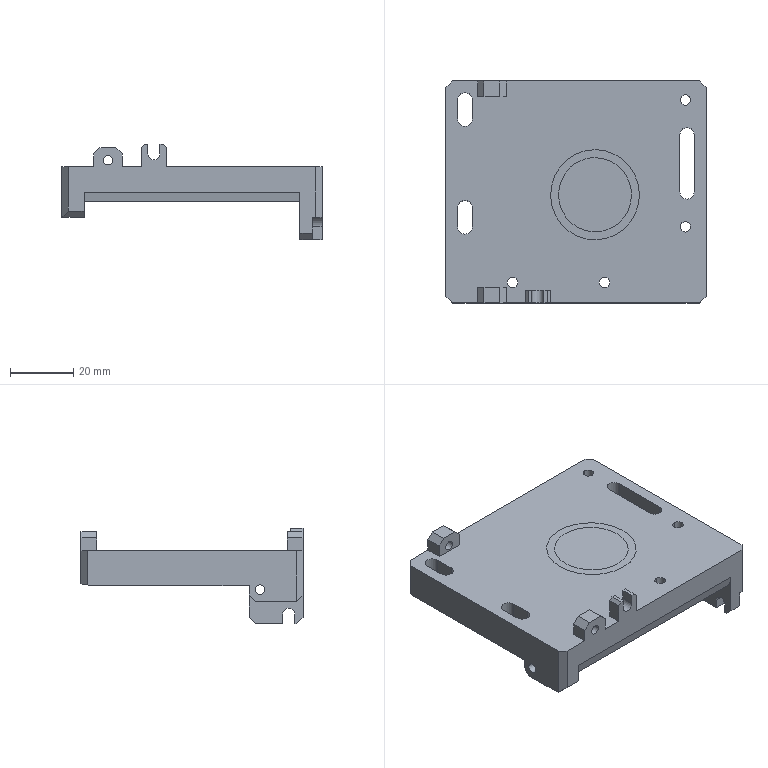NC program | NX | posted with a generic post | part box 82 x 70 x 30 mm
Lines 1 to 2118 of 5501, first 2049 of 2112 lines:
N10 G17 G21 G94 G90
(FLOOR_WALL_COPY , TOOL : D10JING)
N12 T11 M6
N14 G54
N16 G17 G0 G90 X-46. Y40.997 B0. C0. S9500 M3
N18 G43 Z30. H11
N20 Z7.5
N22 G94 G1 Z4.5 F1250.
N24 X-40.
N26 X40.
N28 Y36.122
N30 X-40.
N32 Y31.247
N34 X40.
N36 Y26.373
N38 X-40.
N40 Y21.498
N42 X40.
N44 Y16.623
N46 X-40.
N48 Y11.748
N50 X40.
N52 Y6.873
N54 X-40.
N56 Y1.999
N58 X40.
N60 Y-2.876
N62 X-40.
N64 Y-7.751
N66 X40.
N68 Y-12.626
N70 X-40.
N72 Y-17.501
N74 X40.
N76 Y-22.376
N78 X-40.
N80 Y-27.25
N82 X40.
N84 Y-32.125
N86 X-40.
N88 Y-37.
N90 X40.
N92 X46.
N94 Z7.5
N96 G0 Z30.
N98 X-46. Y40.997
N100 Z7.
N102 G1 Z4.
N104 X-40.
N106 X40.
N108 Y36.122
N110 X-40.
N112 Y31.247
N114 X40.
N116 Y26.373
N118 X-40.
N120 Y21.498
N122 X40.
N124 Y16.623
N126 X-40.
N128 Y11.748
N130 X40.
N132 Y6.873
N134 X-40.
N136 Y1.999
N138 X40.
N140 Y-2.876
N142 X-40.
N144 Y-7.751
N146 X40.
N148 Y-12.626
N150 X-40.
N152 Y-17.501
N154 X40.
N156 Y-22.376
N158 X-40.
N160 Y-27.25
N162 X40.
N164 Y-32.125
N166 X-40.
N168 Y-37.
N170 X40.
N172 X46.
N174 Z7.
N176 G0 Z30.
N178 X-46. Y40.997
N180 Z6.5
N182 G1 Z3.5
N184 X-40.
N186 X40.
N188 Y36.122
N190 X-40.
N192 Y31.247
N194 X40.
N196 Y26.373
N198 X-40.
N200 Y21.498
N202 X40.
N204 Y16.623
N206 X-40.
N208 Y11.748
N210 X40.
N212 Y6.873
N214 X-40.
N216 Y1.999
N218 X40.
N220 Y-2.876
N222 X-40.
N224 Y-7.751
N226 X40.
N228 Y-12.626
N230 X-40.
N232 Y-17.501
N234 X40.
N236 Y-22.376
N238 X-40.
N240 Y-27.25
N242 X40.
N244 Y-32.125
N246 X-40.
N248 Y-37.
N250 X40.
N252 X46.
N254 Z6.5
N256 G0 Z30.
N258 X-46. Y40.997
N260 Z6.
N262 G1 Z3.
N264 X-40.
N266 X40.
N268 Y36.122
N270 X-40.
N272 Y31.247
N274 X40.
N276 Y26.373
N278 X-40.
N280 Y21.498
N282 X40.
N284 Y16.623
N286 X-40.
N288 Y11.748
N290 X40.
N292 Y6.873
N294 X-40.
N296 Y1.999
N298 X40.
N300 Y-2.876
N302 X-40.
N304 Y-7.751
N306 X40.
N308 Y-12.626
N310 X-40.
N312 Y-17.501
N314 X40.
N316 Y-22.376
N318 X-40.
N320 Y-27.25
N322 X40.
N324 Y-32.125
N326 X-40.
N328 Y-37.
N330 X40.
N332 X46.
N334 Z6.
N336 G0 Z30.
N338 X-46. Y40.997
N340 Z5.5
N342 G1 Z2.5
N344 X-40.
N346 X40.
N348 Y36.122
N350 X-40.
N352 Y31.247
N354 X40.
N356 Y26.373
N358 X-40.
N360 Y21.498
N362 X40.
N364 Y16.623
N366 X-40.
N368 Y11.748
N370 X40.
N372 Y6.873
N374 X-40.
N376 Y1.999
N378 X40.
N380 Y-2.876
N382 X-40.
N384 Y-7.751
N386 X40.
N388 Y-12.626
N390 X-40.
N392 Y-17.501
N394 X40.
N396 Y-22.376
N398 X-40.
N400 Y-27.25
N402 X40.
N404 Y-32.125
N406 X-40.
N408 Y-37.
N410 X40.
N412 X46.
N414 Z5.5
N416 G0 Z30.
N418 X-46. Y40.997
N420 Z5.
N422 G1 Z2.
N424 X-40.
N426 X40.
N428 Y36.122
N430 X-40.
N432 Y31.247
N434 X40.
N436 Y26.373
N438 X-40.
N440 Y21.498
N442 X40.
N444 Y16.623
N446 X-40.
N448 Y11.748
N450 X40.
N452 Y6.873
N454 X-40.
N456 Y1.999
N458 X40.
N460 Y-2.876
N462 X-40.
N464 Y-7.751
N466 X40.
N468 Y-12.626
N470 X-40.
N472 Y-17.501
N474 X40.
N476 Y-22.376
N478 X-40.
N480 Y-27.25
N482 X40.
N484 Y-32.125
N486 X-40.
N488 Y-37.
N490 X40.
N492 X46.
N494 Z5.
N496 G0 Z30.
N498 X-46. Y40.997
N500 Z4.5
N502 G1 Z1.5
N504 X-40.
N506 X40.
N508 Y36.122
N510 X-40.
N512 Y31.247
N514 X40.
N516 Y26.373
N518 X-40.
N520 Y21.498
N522 X40.
N524 Y16.623
N526 X-40.
N528 Y11.748
N530 X40.
N532 Y6.873
N534 X-40.
N536 Y1.999
N538 X40.
N540 Y-2.876
N542 X-40.
N544 Y-7.751
N546 X40.
N548 Y-12.626
N550 X-40.
N552 Y-17.501
N554 X40.
N556 Y-22.376
N558 X-40.
N560 Y-27.25
N562 X40.
N564 Y-32.125
N566 X-40.
N568 Y-37.
N570 X40.
N572 X46.
N574 Z4.5
N576 G0 Z30.
N578 X-46. Y40.997
N580 Z4.
N582 G1 Z1.
N584 X-40.
N586 X40.
N588 Y36.122
N590 X-40.
N592 Y31.247
N594 X40.
N596 Y26.373
N598 X-40.
N600 Y21.498
N602 X40.
N604 Y16.623
N606 X-40.
N608 Y11.748
N610 X40.
N612 Y6.873
N614 X-40.
N616 Y1.999
N618 X40.
N620 Y-2.876
N622 X-40.
N624 Y-7.751
N626 X40.
N628 Y-12.626
N630 X-40.
N632 Y-17.501
N634 X40.
N636 Y-22.376
N638 X-40.
N640 Y-27.25
N642 X40.
N644 Y-32.125
N646 X-40.
N648 Y-37.
N650 X40.
N652 X46.
N654 Z4.
N656 G0 Z30.
N658 X-46. Y40.997
N660 Z3.5
N662 G1 Z0.5
N664 X-40.
N666 X40.
N668 Y36.122
N670 X-40.
N672 Y31.247
N674 X40.
N676 Y26.373
N678 X-40.
N680 Y21.498
N682 X40.
N684 Y16.623
N686 X-40.
N688 Y11.748
N690 X40.
N692 Y6.873
N694 X-40.
N696 Y1.999
N698 X40.
N700 Y-2.876
N702 X-40.
N704 Y-7.751
N706 X40.
N708 Y-12.626
N710 X-40.
N712 Y-17.501
N714 X40.
N716 Y-22.376
N718 X-40.
N720 Y-27.25
N722 X40.
N724 Y-32.125
N726 X-40.
N728 Y-37.
N730 X40.
N732 X46.
N734 Z3.5
N736 G0 Z30.
N738 X-46. Y40.997
N740 Z3.
N742 G1 Z0.
N744 X-40.
N746 X40.
N748 Y36.122
N750 X-40.
N752 Y31.247
N754 X40.
N756 Y26.373
N758 X-40.
N760 Y21.498
N762 X40.
N764 Y16.623
N766 X-40.
N768 Y11.748
N770 X40.
N772 Y6.873
N774 X-40.
N776 Y1.999
N778 X40.
N780 Y-2.876
N782 X-40.
N784 Y-7.751
N786 X40.
N788 Y-12.626
N790 X-40.
N792 Y-17.501
N794 X40.
N796 Y-22.376
N798 X-40.
N800 Y-27.25
N802 X40.
N804 Y-32.125
N806 X-40.
N808 Y-37.
N810 X40.
N812 X46.
N814 Z3.
N816 G0 Z30.
N818 M5
(CAVITY_MILL_COPY_1 , TOOL : D10)
N820 T10 M6
N822 G54
N824 G17 G0 G90 X41.997 Y4.33 B0. C0. S9500 M3
N826 G43 Z30. H10
N828 Z1.05
N830 G94 G1 Z-0.45 F1000.
N832 X35.997 Y0.866
N834 G3 X35.497 Y0. R1.
N836 G1 X5.497
N838 Y11.496 F3000.
N840 X4.071
N842 X4.1 Y8.486
N844 G2 X-2.181 Y-11.496 R35.259
N846 G1 X5.497
N848 Y0.
N850 X11.497
N852 Y17.496
N854 X-1.972
N856 G2 X-1.9 Y15.462 R29.147
N858 G1 Y13.9
N860 G2 X-1.961 Y12.024 R29.1
N862 X-1.93 Y11.498 R29.278
N864 G1 X-1.9 Y8.469
N866 G2 X-11.497 Y-13.078 R29.259
N868 G1 Y-17.496
N870 X11.497
N872 Y0.
N874 X17.497
N876 Y23.496
N878 X-9.345
N880 G2 X-7.9 Y15.459 R23.147
N882 G1 Y13.9
N884 G2 X-7.977 Y12.015 R23.1
N886 X-7.922 Y11.2 R23.278
N888 G1 X-7.916 Y11.069
N890 X-7.9 Y8.494
N892 G2 X-16.153 Y-9.18 R23.259
N894 X-17.497 Y-10.232 R22.932
N896 G1 Y-23.496
N898 X17.497
N900 Y0.
N902 X23.497
N904 Y29.496
N906 X-21.219
N908 G2 X-13.9 Y15.455 R17.147
N910 G1 Y13.9
N912 G2 X-14.005 Y12.006 R17.1
N914 X-13.915 Y10.902 R17.278
N916 G1 X-13.9 Y8.493
N918 G2 X-20.024 Y-4.596 R17.259
N920 X-23.497 Y-6.864 R16.932
N922 G1 Y-29.496
N924 X23.497
N926 Y0.
N928 X29.497
N930 Y35.496
N932 X-29.497
N934 Y26.483
N936 G2 X-19.9 Y15.453 R11.147
N938 G1 Y13.9
N940 G2 X-20.064 Y11.999 R11.1
N942 X-19.907 Y10.604 R11.278
N944 G1 X-19.9 Y10.456
N946 Y8.527
N948 G2 X-23.895 Y-0.012 R11.259
N950 X-29.497 Y-2.495 R10.932
N952 G1 Y-35.496
N954 X29.497
N956 Y0.
N958 X35.497
N960 Y41.002
N962 G3 X35.003 Y41.496 R0.494
N964 G1 X-35.003
N966 G3 X-35.497 Y41.002 R0.494
N968 G1 Y21.775
N970 G3 X-38.463 Y20.749 R6.117
N972 X-39.997 Y19.298 R6.424
N974 G1 Y16.451
N976 G2 X-37.793 Y19.754 R5.224
N978 X-35.047 Y20.591 R4.917
N980 G1 X-31.
N982 G2 X-25.9 Y15.45 R5.147
N984 G1 Y13.9
N986 G2 X-26.218 Y12.128 R5.1
N988 G1 X-26.268 Y11.998
N990 G2 X-25.9 Y10.307 R5.278
N992 G1 Y8.55
N994 G2 X-27.766 Y4.572 R5.259
N996 X-30.948 Y3.409 R4.932
N998 G1 X-35.
N1000 G2 X-39.997 Y7.524 R5.137
N1002 G1 Y4.697
N1004 G3 X-35.497 Y2.231 R6.337
N1006 G1 Y-41.002
N1008 G3 X-35.003 Y-41.496 R0.494
N1010 G1 X35.003
N1012 G3 X35.497 Y-41.002 R0.494
N1014 G1 Y0.
N1016 G2 X35.997 Y0.866 R1.
N1018 G1 X41.997 Y4.33
N1020 Z1.05
N1022 G0 Z0.6
N1024 G1 Z-0.9 F1000.
N1026 X35.997 Y0.866
N1028 G3 X35.497 Y0. R1.
N1030 G1 X5.497
N1032 Y11.496 F3000.
N1034 X4.069
N1036 X4.1 Y8.201
N1038 G2 X-1.866 Y-11.496 R35.121
N1040 G1 X5.497
N1042 Y0.
N1044 X11.497
N1046 Y17.496
N1048 X-1.943
N1050 G2 X-1.9 Y15.864 R29.121
N1052 G1 Y13.9
N1054 G2 X-1.961 Y12.023 R29.1
N1056 X-1.932 Y11.548 R29.386
N1058 G1 X-1.9 Y8.165
N1060 G2 X-11.497 Y-13.52 R29.121
N1062 G1 Y-17.496
N1064 X11.497
N1066 Y0.
N1068 X17.497
N1070 Y23.496
N1072 X-9.179
N1074 G2 X-7.9 Y15.869 R23.121
N1076 G1 Y13.9
N1078 G2 X-7.977 Y12.013 R23.1
N1080 X-7.924 Y11.238 R23.386
N1082 G1 X-7.917 Y11.1
N1084 X-7.9 Y8.149
N1086 G2 X-17.497 Y-10.667 R23.121
N1088 G1 Y-23.496
N1090 X17.497
N1092 Y0.
N1094 X23.497
N1096 Y29.496
N1098 X-20.598
N1100 G2 X-13.9 Y15.875 R17.121
N1102 G1 Y13.9
N1104 G2 X-14.005 Y12.004 R17.1
N1106 X-13.916 Y10.927 R17.386
N1108 G1 X-13.9 Y8.125
N1110 G2 X-23.497 Y-7.292 R17.121
N1112 G1 Y-29.496
N1114 X23.497
N1116 Y0.
N1118 X29.497
N1120 Y35.496
N1122 X-29.497
N1124 Y26.929
N1126 G2 X-19.9 Y15.883 R11.121
N1128 G1 Y13.9
N1130 G2 X-20.064 Y11.997 R11.1
N1132 X-19.908 Y10.617 R11.386
N1134 G1 X-19.9 Y10.462
N1136 Y8.117
N1138 G2 X-29.497 Y-2.929 R11.121
N1140 G1 Y-35.496
N1142 X29.497
N1144 Y0.
N1146 X35.497
N1148 Y41.002
N1150 G3 X35.003 Y41.496 R0.494
N1152 G1 X-35.003
N1154 G3 X-35.497 Y41.002 R0.494
N1156 G1 Y22.213
N1158 G3 X-39.997 Y19.757 R6.321
N1160 G1 Y16.934
N1162 G2 X-35. Y21.034 R5.121
N1164 G1 X-31.
N1166 G2 X-25.9 Y15.893 R5.121
N1168 G1 Y13.9
N1170 G2 X-26.262 Y12.014 R5.1
N1172 G1 Y11.987
N1174 G2 X-25.9 Y10.307 R5.386
N1176 G1 Y8.107
N1178 G2 X-31. Y2.966 R5.121
N1180 G1 X-35.
N1182 G2 X-39.997 Y7.08 R5.136
N1184 G1 Y4.254
N1186 G3 X-35.497 Y1.788 R6.336
N1188 G1 Y-41.002
N1190 G3 X-35.003 Y-41.496 R0.494
N1192 G1 X35.003
N1194 G3 X35.497 Y-41.002 R0.494
N1196 G1 Y0.
N1198 G2 X35.997 Y0.866 R1.
N1200 G1 X41.997 Y4.33
N1202 Z0.6
N1204 G0 Y-2.199 Z0.1
N1206 G1 Z-1.4 F1000.
N1208 X35.997 Y-5.663
N1210 G3 X35.497 Y-6.529 R1.
N1212 G1 X5.497
N1214 Y-1.562 F3000.
N1216 G2 X3.341 Y0.74 R35.121
N1218 X-1.812 Y-11.496 R35.1
N1220 G1 X5.497
N1222 Y-6.529
N1224 X11.497
N1226 Y1.109
N1228 G2 X1.542 Y17.496 R29.121
N1230 G1 X-1.548
N1232 G2 X-1.9 Y16.036 R29.188
N1234 G1 Y13.9
N1236 G2 X-1.961 Y12.024 R29.1
N1238 X-1.931 Y11.532 R29.366
N1240 G1 X-1.917 Y11.258
N1242 X-1.9 Y8.034
N1244 G2 X-11.497 Y-13.598 R29.1
N1246 G1 Y-17.496
N1248 X11.497
N1250 Y-6.529
N1252 X17.497
N1254 Y4.144
N1256 G2 X6.9 Y23.496 R23.121
N1258 G1 X-6.9
N1260 G2 X-7.915 Y16.826 R23.188
N1262 X-7.9 Y16. R23.1
N1264 G1 Y13.9
N1266 G2 X-7.977 Y12.014 R23.1
N1268 X-7.923 Y11.226 R23.366
N1270 G1 X-7.916 Y11.089
N1272 X-7.9 Y8.016
N1274 G2 X-17.497 Y-10.743 R23.1
N1276 G1 Y-23.496
N1278 X17.497
N1280 Y-6.529
N1282 X23.497
N1284 Y7.75
N1286 G2 X12.9 Y23.617 R17.121
N1288 G1 Y29.383
N1290 Y29.496
N1292 X-12.9
N1294 Y29.383
N1296 Y23.589
N1298 G2 X-13.977 Y17.622 R17.188
N1300 X-13.9 Y16. R17.1
N1302 G1 Y13.9
N1304 G2 X-14.005 Y12.005 R17.1
N1306 X-13.916 Y10.919 R17.366
N1308 G1 X-13.9 Y8.
N1310 G2 X-23.497 Y-7.366 R17.1
N1312 G1 Y-29.496
N1314 X23.497
N1316 Y-6.529
N1318 X29.497
N1320 Y12.471
N1322 G2 X18.9 Y23.61 R11.121
N1324 G1 Y29.47
N1326 G2 X20.706 Y35.496 R11.121
N1328 G1 X-20.706
N1330 G2 X-18.9 Y29.39 R11.121
N1332 G1 Y23.594
N1334 G2 X-20.17 Y18.433 R11.188
N1336 X-19.9 Y16. R11.1
N1338 G1 Y13.9
N1340 G2 X-20.064 Y11.998 R11.1
N1342 X-19.908 Y10.613 R11.366
N1344 G1 X-19.9 Y10.46
N1346 Y8.
N1348 G2 X-29.497 Y-2.998 R11.1
N1350 G1 Y-35.496
N1352 X29.497
N1354 Y-6.529
N1356 X35.497
N1358 Y17.28
N1360 G3 X39.997 Y19.736 R6.321
N1362 G1 Y22.559
N1364 G2 X35. Y18.459 R5.121
N1366 G1 X30.
N1368 G2 X24.9 Y23.6 R5.121
N1370 G1 Y29.4
N1372 G2 X30. Y34.541 R5.121
N1374 G1 X35.
N1376 G2 X39.997 Y30.441 R5.121
N1378 G1 Y33.264
N1380 G3 X35.497 Y35.72 R6.321
N1382 G1 Y41.002
N1384 G3 X35.003 Y41.496 R0.494
N1386 G1 X-35.003
N1388 G3 X-35.497 Y41.002 R0.494
N1390 G1 Y35.72
N1392 G3 X-39.997 Y33.264 R6.321
N1394 G1 Y30.441
N1396 G2 X-35. Y34.541 R5.121
N1398 G1 X-30.
N1400 G2 X-24.9 Y29.4 R5.121
N1402 G1 Y23.6
N1404 G2 X-27.144 Y19.338 R5.188
N1406 X-25.9 Y16. R5.1
N1408 G1 Y13.9
N1410 G2 X-26.261 Y12.015 R5.1
N1412 G1 Y11.986
N1414 G2 X-25.9 Y10.307 R5.366
N1416 G1 Y8.
N1418 G2 X-31. Y2.9 R5.1
N1420 G1 X-35.
N1422 G2 X-39.997 Y6.982 R5.1
N1424 G1 Y4.164
N1426 G3 X-35.497 Y1.72 R6.3
N1428 G1 Y-41.002
N1430 G3 X-35.003 Y-41.496 R0.494
N1432 G1 X35.003
N1434 G3 X35.497 Y-41.002 R0.494
N1436 G1 Y-6.529
N1438 G2 X35.997 Y-5.663 R1.
N1440 G1 X41.997 Y-2.199
N1442 Z0.1
N1444 G0 Y-2.449 Z-0.4
N1446 G1 Z-1.9 F1000.
N1448 X35.997 Y-5.913
N1450 G3 X35.497 Y-6.779 R1.
N1452 G1 X5.497
N1454 Y-2.062 F3000.
N1456 G2 X3.254 Y0.341 R35.121
N1458 X-1.813 Y-11.496 R35.1
N1460 G1 X5.497
N1462 Y-6.779
N1464 X11.497
N1466 Y0.609
N1468 G2 X1.44 Y17.496 R29.121
N1470 G1 X-1.446
N1472 G2 X-1.9 Y15.541 R29.223
N1474 G1 Y13.9
N1476 G2 X-1.961 Y12.024 R29.1
N1478 X-1.931 Y11.517 R29.347
N1480 G1 X-1.917 Y11.246
N1482 X-1.9 Y8.033
N1484 G2 X-11.497 Y-13.598 R29.1
N1486 G1 Y-17.496
N1488 X11.497
N1490 Y-6.779
N1492 X17.497
N1494 Y3.644
N1496 G2 X6.9 Y23.123 R23.121
N1498 G1 Y23.496
N1500 X-6.9
N1502 Y23.065
N1504 G2 X-7.903 Y16.369 R23.223
N1506 X-7.9 Y16. R23.1
N1508 G1 Y13.9
N1510 G2 X-7.977 Y12.014 R23.1
N1512 X-7.923 Y11.214 R23.347
N1514 G1 X-7.916 Y11.079
N1516 X-7.9 Y8.016
N1518 G2 X-17.497 Y-10.743 R23.1
N1520 G1 Y-23.496
N1522 X17.497
N1524 Y-6.779
N1526 X23.497
N1528 Y7.25
N1530 G2 X12.9 Y23.117 R17.121
N1532 G1 Y29.496
N1534 X-12.9
N1536 Y23.08
N1538 G2 X-13.943 Y17.217 R17.223
N1540 X-13.9 Y16. R17.1
N1542 G1 Y13.9
N1544 G2 X-14.005 Y12.006 R17.1
N1546 X-13.915 Y10.912 R17.347
N1548 G1 X-13.9 Y8.
N1550 G2 X-23.497 Y-7.366 R17.1
N1552 G1 Y-29.496
N1554 X23.497
N1556 Y-6.779
N1558 X29.497
N1560 Y11.971
N1562 G2 X18.9 Y23.11 R11.121
N1564 G1 Y29.89
N1566 G2 X20.399 Y35.496 R11.121
N1568 G1 X-20.399
N1570 G2 X-18.9 Y29.89 R11.121
N1572 G1 Y23.088
N1574 G2 X-20.096 Y18.078 R11.223
N1576 X-19.9 Y16. R11.1
N1578 G1 Y13.9
N1580 G2 X-20.064 Y11.999 R11.1
N1582 X-19.908 Y10.609 R11.347
N1584 G1 X-19.9 Y10.458
N1586 Y8.
N1588 G2 X-29.497 Y-2.998 R11.1
N1590 G1 Y-35.496
N1592 X29.497
N1594 Y-6.779
N1596 X35.497
N1598 Y16.78
N1600 G3 X39.997 Y19.241 R6.328
N1602 G1 Y22.066
N1604 G2 X35. Y17.959 R5.128
N1606 G1 X30.
N1608 G2 X24.9 Y23.1 R5.121
N1610 G1 Y29.9
N1612 G2 X30. Y35.041 R5.121
N1614 G1 X35.
N1616 G2 X39.997 Y30.934 R5.128
N1618 G1 Y33.759
N1620 G3 X35.497 Y36.22 R6.328
N1622 G1 Y41.002
N1624 G3 X35.003 Y41.496 R0.494
N1626 G1 X-35.003
N1628 G3 X-35.497 Y41.002 R0.494
N1630 G1 Y36.22
N1632 G3 X-39.997 Y33.759 R6.328
N1634 G1 Y30.934
N1636 G2 X-35. Y35.041 R5.128
N1638 G1 X-30.
N1640 G2 X-24.9 Y29.9 R5.121
N1642 G1 Y23.1
N1644 G2 X-26.889 Y19.019 R5.223
N1646 X-25.9 Y16. R5.1
N1648 G1 Y13.9
N1650 G2 X-26.26 Y12.017 R5.1
N1652 G1 Y11.984
N1654 G2 X-25.9 Y10.307 R5.347
N1656 G1 Y8.
N1658 G2 X-31. Y2.9 R5.1
N1660 G1 X-35.
N1662 G2 X-39.997 Y6.982 R5.1
N1664 G1 Y4.164
N1666 G3 X-35.497 Y1.72 R6.3
N1668 G1 Y-41.002
N1670 G3 X-35.003 Y-41.496 R0.494
N1672 G1 X35.003
N1674 G3 X35.497 Y-41.002 R0.494
N1676 G1 Y-6.779
N1678 G2 X35.997 Y-5.913 R1.
N1680 G1 X41.997 Y-2.449
N1682 Z-0.4
N1684 G0 Y-2.699 Z-0.9
N1686 G1 Z-2.4 F1000.
N1688 X35.997 Y-6.163
N1690 G3 X35.497 Y-7.029 R1.
N1692 G1 X5.497
N1694 Y-2.562 F3000.
N1696 G2 X3.164 Y-0.052 R35.121
N1698 X-1.813 Y-11.496 R35.1
N1700 G1 X5.497
N1702 Y-7.029
N1704 X11.497
N1706 Y0.109
N1708 G2 X1.347 Y17.496 R29.121
N1710 G1 X-1.355
N1712 G2 X-1.9 Y15.05 R29.276
N1714 G1 Y13.9
N1716 G2 X-1.96 Y12.025 R29.1
N1718 X-1.929 Y11.495 R29.31
N1720 G1 X-1.916 Y11.228
N1722 X-1.9 Y8.032
N1724 G2 X-11.497 Y-13.598 R29.1
N1726 G1 Y-17.496
N1728 X11.497
N1730 Y-7.029
N1732 X17.497
N1734 Y3.144
N1736 G2 X6.9 Y22.623 R23.121
N1738 G1 Y23.496
N1740 X-6.9
N1742 Y22.537
N1744 G2 X-7.9 Y15.888 R23.276
N1746 G1 Y13.9
N1748 G2 X-7.977 Y12.015 R23.1
N1750 X-7.922 Y11.198 R23.31
N1752 G1 X-7.915 Y11.065
N1754 X-7.9 Y8.015
N1756 G2 X-17.497 Y-10.743 R23.1
N1758 G1 Y-23.496
N1760 X17.497
N1762 Y-7.029
N1764 X23.497
N1766 Y6.75
N1768 G2 X12.9 Y22.617 R17.121
N1770 G1 Y29.496
N1772 X-12.9
N1774 Y22.563
N1776 G2 X-13.918 Y16.793 R17.276
N1778 X-13.9 Y16. R17.1
N1780 G1 Y13.9
N1782 G2 X-14.005 Y12.007 R17.1
N1784 X-13.915 Y10.901 R17.31
N1786 G1 X-13.9 Y8.
N1788 G2 X-23.497 Y-7.366 R17.1
N1790 G1 Y-29.496
N1792 X23.497
N1794 Y-7.029
N1796 X29.497
N1798 Y11.471
N1800 G2 X18.9 Y22.61 R11.121
N1802 G1 Y30.39
N1804 G2 X20.126 Y35.496 R11.121
N1806 G1 X-20.126
N1808 G2 X-18.9 Y30.39 R11.121
N1810 G1 Y22.579
N1812 G2 X-20.033 Y17.711 R11.276
N1814 X-19.9 Y16. R11.1
N1816 G1 Y13.9
N1818 G2 X-20.064 Y12. R11.1
N1820 X-19.907 Y10.604 R11.31
N1822 G1 X-19.9 Y10.455
N1824 Y8.
N1826 G2 X-29.497 Y-2.998 R11.1
N1828 G1 Y-35.496
N1830 X29.497
N1832 Y-7.029
N1834 X35.497
N1836 Y16.281
N1838 G3 X39.997 Y18.749 R6.341
N1840 G1 Y21.578
N1842 G2 X35. Y17.459 R5.141
N1844 G1 X29.983
N1846 G2 X24.9 Y22.6 R5.121
N1848 G1 Y30.4
N1850 G2 X30. Y35.541 R5.121
N1852 G1 X35.
N1854 G2 X39.997 Y31.422 R5.141
N1856 G1 Y34.251
N1858 G3 X35.497 Y36.719 R6.341
N1860 G1 Y41.002
N1862 G3 X35.003 Y41.496 R0.494
N1864 G1 X-35.003
N1866 G3 X-35.497 Y41.002 R0.494
N1868 G1 Y36.718
N1870 G3 X-39.997 Y34.243 R6.352
N1872 G1 Y31.413
N1874 G2 X-35. Y35.541 R5.152
N1876 G1 X-30.
N1878 G2 X-24.9 Y30.4 R5.121
N1880 G1 Y22.6
N1882 G2 X-26.67 Y18.695 R5.276
N1884 X-25.9 Y16. R5.1
N1886 G1 Y13.9
N1888 G2 X-26.261 Y12.016 R5.1
N1890 G1 Y11.985
N1892 G2 X-25.9 Y10.307 R5.31
N1894 G1 Y8.
N1896 G2 X-31. Y2.9 R5.1
N1898 G1 X-35.
N1900 G2 X-39.997 Y6.983 R5.1
N1902 G1 Y4.164
N1904 G3 X-35.497 Y1.72 R6.3
N1906 G1 Y-41.002
N1908 G3 X-35.003 Y-41.496 R0.494
N1910 G1 X35.003
N1912 G3 X35.497 Y-41.002 R0.494
N1914 G1 Y-7.029
N1916 G2 X35.997 Y-6.163 R1.
N1918 G1 X41.997 Y-2.699
N1920 Z-0.9
N1922 G0 X41.998 Y-2.949 Z-1.4
N1924 G1 Z-2.9 F1000.
N1926 X35.998 Y-6.413
N1928 G3 X35.498 Y-7.279 R1.
N1930 G1 X5.498
N1932 Y-3.062 F3000.
N1934 G2 X3.07 Y-0.44 R35.121
N1936 X-1.813 Y-11.496 R35.1
N1938 G1 X5.498
N1940 Y-7.279
N1942 X11.498
N1944 Y-0.391
N1946 G2 X1.263 Y17.496 R29.121
N1948 G1 X-1.265
N1950 G2 X-1.9 Y14.525 R29.169
N1952 G1 Y13.9
N1954 G2 X-1.96 Y12.025 R29.1
N1956 X-1.929 Y11.486 R29.308
N1958 G1 X-1.923 Y11.359
N1960 X-1.9 Y8.02
N1962 G2 X-11.498 Y-13.598 R29.1
N1964 G1 Y-17.496
N1966 X11.498
N1968 Y-7.279
N1970 X17.498
N1972 Y2.644
N1974 G2 X6.9 Y22.123 R23.121
N1976 G1 Y23.496
N1978 X-6.9
N1980 Y22.104
N1982 G2 X-7.9 Y15.364 R23.169
N1984 G1 Y13.9
N1986 G2 X-7.977 Y12.016 R23.1
N1988 X-7.922 Y11.191 R23.308
N1990 G1 X-7.9 Y8.
N1992 G2 X-17.498 Y-10.743 R23.1
N1994 G1 Y-23.496
N1996 X17.498
N1998 Y-7.279
N2000 X23.498
N2002 Y6.25
N2004 G2 X12.9 Y22.117 R17.121
N2006 G1 Y29.496
N2008 X-12.9
N2010 Y22.103
N2012 G2 X-13.903 Y16.315 R17.169
N2014 X-13.9 Y16. R17.1
N2016 G1 Y13.9
N2018 G2 X-14.005 Y12.007 R17.1
N2020 X-13.915 Y10.896 R17.308
N2022 G1 X-13.9 Y10.602
N2024 Y8.
N2026 G2 X-23.498 Y-7.366 R17.1
N2028 G1 Y-29.496
N2030 X23.498
N2032 Y-7.279
N2034 X29.498
N2036 Y10.971
N2038 G2 X18.9 Y22.11 R11.121
N2040 G1 Y30.89
N2042 G2 X19.885 Y35.496 R11.121
N2044 G1 X-19.885
N2046 G2 X-18.9 Y30.89 R11.121
N2048 G1 Y22.101
N2050 G2 X-19.978 Y17.311 R11.169
N2052 X-19.9 Y16. R11.1
N2054 G1 Y13.9
N2056 G2 X-20.064 Y12. R11.1
N2058 X-19.907 Y10.602 R11.308
N2060 G1 X-19.9 Y10.454
N2062 Y8.
N2064 G2 X-29.498 Y-2.998 R11.1
N2066 G1 Y-35.496
N2068 X29.498
N2070 Y-7.279
N2072 X35.498
N2074 Y15.78
N2076 G3 X39.998 Y18.236 R6.321
N2078 G1 Y21.06
N2080 G2 X35. Y16.959 R5.121
N2082 G1 X30.
N2084 G2 X24.9 Y22.1 R5.121
N2086 G1 Y30.9
N2088 G2 X30. Y36.041 R5.121
N2090 G1 X35.
N2092 G2 X39.998 Y31.94 R5.121
N2094 G1 Y34.764
N2096 G3 X35.498 Y37.22 R6.321
N2098 G1 Y41.002
N2100 G3 X35.003 Y41.496 R0.494
N2102 G1 X-35.003
N2104 G3 X-35.498 Y41.002 R0.494
N2106 G1 Y37.22
N2108 G3 X-39.998 Y34.764 R6.321
N2110 G1 Y31.94
N2112 G2 X-35. Y36.041 R5.121
N2114 G1 X-30.
N2116 G2 X-24.9 Y30.9 R5.121
N2118 G1 Y22.1
N2120 G2 X-26.485 Y18.372 R5.169
N2122 X-25.9 Y16. R5.1
N2124 G1 Y13.9
N2126 G2 X-26.26 Y12.017 R5.1
N2128 G1 Y11.985
N2130 G2 X-25.9 Y10.307 R5.308
N2132 G1 Y8.
N2134 G2 X-31. Y2.9 R5.1
N2136 G1 X-35.
N2138 G2 X-39.998 Y6.983 R5.1
N2140 G1 Y4.164
N2142 G3 X-35.498 Y1.72 R6.3
N2144 G1 Y-41.002
N2146 G3 X-35.003 Y-41.496 R0.494
N2148 G1 X35.003
N2150 G3 X35.498 Y-41.002 R0.494
N2152 G1 Y-7.279
N2154 G2 X35.998 Y-6.413 R1.
N2156 G1 X41.998 Y-2.949
N2158 Z-1.4
N2160 G0 Y-2.984 Z-1.9
N2162 G1 Z-3.4 F1000.
N2164 X35.998 Y-6.448
N2166 G3 X35.498 Y-7.314 R1.
N2168 G1 X5.498
N2170 Y-3.132 F3000.
N2172 G2 X3.056 Y-0.496 R35.1
N2174 X-1.813 Y-11.496 R35.1
N2176 G1 X5.498
N2178 Y-7.314
N2180 X11.498
N2182 Y-0.46
N2184 G2 X1.251 Y17.496 R29.1
N2186 G1 X-1.251
N2188 G2 X-1.9 Y14.436 R29.1
N2190 G1 Y14.014
N2192 G2 X-1.955 Y12.021 R28.962
N2194 X-1.9 Y10.455 R28.694
N2196 G1 Y8.
N2198 G2 X-11.498 Y-13.598 R29.1
N2200 G1 Y-17.496
N2202 X11.498
N2204 Y-7.314
N2206 X17.498
N2208 Y2.576
N2210 G2 X6.9 Y22. R23.1
N2212 G1 Y23.496
N2214 X-6.9
N2216 Y22.
N2218 G2 X-7.901 Y15.274 R23.1
N2220 G1 X-7.9 Y13.991
N2222 G2 X-7.97 Y12.02 R22.962
N2224 X-7.9 Y10.428 R22.694
N2226 G1 Y8.
N2228 G2 X-17.498 Y-10.743 R23.1
N2230 G1 Y-23.496
N2232 X17.498
N2234 Y-7.314
N2236 X23.498
N2238 Y6.185
N2240 G2 X12.9 Y22. R17.1
N2242 G1 Y29.496
N2244 X-12.9
N2246 Y22.
N2248 G2 X-13.902 Y16.234 R17.1
N2250 G1 X-13.9 Y13.966
N2252 G2 X-13.996 Y12.017 R16.962
N2254 X-13.9 Y10.397 R16.694
N2256 G1 Y8.
N2258 G2 X-23.498 Y-7.366 R17.1
N2260 G1 Y-29.496
N2262 X23.498
N2264 Y-7.314
N2266 X29.498
N2268 Y10.911
N2270 G2 X18.9 Y22. R11.1
N2272 G1 Y31.
N2274 G2 X19.851 Y35.496 R11.1
N2276 G1 X-19.851
N2278 G2 X-18.9 Y31. R11.1
N2280 G1 Y22.
N2282 G2 X-19.97 Y17.245 R11.1
N2284 X-19.9 Y16. R11.1
N2286 G1 Y13.938
N2288 G2 X-20.05 Y12.013 R10.962
N2290 X-19.9 Y10.359 R10.694
N2292 G1 Y8.
N2294 G2 X-29.498 Y-2.998 R11.1
N2296 G1 Y-35.496
N2298 X29.498
N2300 Y-7.314
N2302 X35.498
N2304 Y15.72
N2306 G3 X39.998 Y18.164 R6.3
N2308 G1 Y20.983
N2310 G2 X35. Y16.9 R5.1
N2312 G1 X30.
N2314 G2 X24.9 Y22. R5.1
N2316 G1 Y31.
N2318 G2 X30. Y36.1 R5.1
N2320 G1 X35.
N2322 G2 X39.998 Y32.017 R5.1
N2324 G1 Y34.836
N2326 G3 X35.498 Y37.28 R6.3
N2328 G1 Y41.002
N2330 G3 X35.003 Y41.496 R0.494
N2332 G1 X-35.003
N2334 G3 X-35.498 Y41.002 R0.494
N2336 G1 Y37.28
N2338 G3 X-39.998 Y34.836 R6.3
N2340 G1 Y32.017
N2342 G2 X-35. Y36.1 R5.1
N2344 G1 X-30.
N2346 G2 X-24.9 Y31. R5.1
N2348 G1 Y22.
N2350 G2 X-26.462 Y18.327 R5.1
N2352 X-25.9 Y16. R5.1
N2354 G1 Y13.9
N2356 G2 X-26.247 Y11.998 R4.962
N2358 X-25.9 Y10.307 R4.694
N2360 G1 Y8.
N2362 G2 X-31. Y2.9 R5.1
N2364 G1 X-35.
N2366 G2 X-39.998 Y6.983 R5.1
N2368 G1 Y4.164
N2370 G3 X-35.498 Y1.72 R6.3
N2372 G1 Y-41.002
N2374 G3 X-35.003 Y-41.496 R0.494
N2376 G1 X35.003
N2378 G3 X35.498 Y-41.002 R0.494
N2380 G1 Y-7.314
N2382 G2 X35.998 Y-6.448 R1.
N2384 G1 X41.998 Y-2.984
N2386 Z-1.9
N2388 G0 Z-2.4
N2390 G1 Z-3.9 F1000.
N2392 X35.998 Y-6.448
N2394 G3 X35.498 Y-7.314 R1.
N2396 G1 X5.498
N2398 Y-3.133 F3000.
N2400 G2 X3.056 Y-0.496 R35.1
N2402 X-1.813 Y-11.496 R35.1
N2404 G1 X5.498
N2406 Y-7.314
N2408 X11.498
N2410 Y-0.46
N2412 G2 X1.251 Y17.496 R29.1
N2414 G1 X-1.251
N2416 G2 X-1.902 Y14.429 R29.1
N2418 G1 X-1.903 Y13.013
N2420 G2 X-1.935 Y12.149 R29.554
N2422 G1 X-1.9 Y11.801
N2424 Y8.
N2426 G2 X-11.498 Y-13.598 R29.1
N2428 G1 Y-17.496
N2430 X11.498
N2432 Y-7.314
N2434 X17.498
N2436 Y2.576
N2438 G2 X6.9 Y22. R23.1
N2440 G1 Y23.496
N2442 X-6.9
N2444 Y22.
N2446 G2 X-7.902 Y15.271 R23.1
N2448 G1 X-7.903 Y13.091
N2450 G2 X-7.954 Y12.027 R23.554
N2452 G1 X-7.9 Y11.496
N2454 Y8.
N2456 G2 X-17.498 Y-10.743 R23.1
N2458 G1 Y-23.496
N2460 X17.498
N2462 Y-7.314
N2464 X23.498
N2466 Y6.185
N2468 G2 X12.9 Y22. R17.1
N2470 G1 Y29.496
N2472 X-12.9
N2474 Y22.
N2476 G2 X-13.902 Y16.234 R17.1
N2478 G1 X-13.903 Y13.18
N2480 G2 X-13.98 Y11.972 R17.554
N2482 G1 X-13.9 Y11.191
N2484 Y8.
N2486 G2 X-23.498 Y-7.366 R17.1
N2488 G1 Y-29.496
N2490 X23.498
N2492 Y-7.314
N2494 X29.498
N2496 Y10.911
N2498 G2 X18.9 Y22. R11.1
N2500 G1 Y31.
N2502 G2 X19.851 Y35.496 R11.1
N2504 G1 X-19.851
N2506 G2 X-18.9 Y31. R11.1
N2508 G1 Y22.
N2510 G2 X-19.97 Y17.245 R11.1
N2512 X-19.9 Y16. R11.1
N2514 G1 Y13.356
N2516 G2 X-20.027 Y11.955 R11.554
N2518 X-19.93 Y11.19 R15.951
N2520 G1 X-19.9 Y10.889
N2522 Y8.
N2524 G2 X-29.498 Y-2.998 R11.1
N2526 G1 Y-35.496
N2528 X29.498
N2530 Y-7.314
N2532 X35.498
N2534 Y15.72
N2536 G3 X39.998 Y18.164 R6.3
N2538 G1 Y20.983
N2540 G2 X35. Y16.9 R5.1
N2542 G1 X30.
N2544 G2 X24.9 Y22. R5.1
N2546 G1 Y31.
N2548 G2 X30. Y36.1 R5.1
N2550 G1 X35.
N2552 G2 X39.998 Y32.017 R5.1
N2554 G1 Y34.836
N2556 G3 X35.498 Y37.28 R6.3
N2558 G1 Y41.002
N2560 G3 X35.003 Y41.496 R0.495
N2562 G1 X-35.003
N2564 G3 X-35.498 Y41.002 R0.495
N2566 G1 Y37.28
N2568 G3 X-39.998 Y34.836 R6.3
N2570 G1 Y32.017
N2572 G2 X-35. Y36.1 R5.1
N2574 G1 X-30.
N2576 G2 X-24.9 Y31. R5.1
N2578 G1 Y22.
N2580 G2 X-26.462 Y18.327 R5.1
N2582 X-25.9 Y16. R5.1
N2584 G1 Y13.472
N2586 G2 X-26.152 Y12.021 R5.554
N2588 X-25.9 Y10.586 R9.951
N2590 G1 Y8.
N2592 G2 X-31. Y2.9 R5.1
N2594 G1 X-35.
N2596 G2 X-39.998 Y6.983 R5.1
N2598 G1 Y4.164
N2600 G3 X-35.498 Y1.72 R6.3
N2602 G1 Y-41.002
N2604 G3 X-35.003 Y-41.496 R0.495
N2606 G1 X35.003
N2608 G3 X35.498 Y-41.002 R0.495
N2610 G1 Y-7.314
N2612 G2 X35.998 Y-6.448 R1.
N2614 G1 X41.998 Y-2.984
N2616 Z-2.4
N2618 G0 Z-2.9
N2620 G1 Z-4.4 F1000.
N2622 X35.998 Y-6.448
N2624 G3 X35.498 Y-7.315 R1.
N2626 G1 X5.498
N2628 Y-3.133 F3000.
N2630 G2 X3.056 Y-0.496 R35.1
N2632 X-1.813 Y-11.496 R35.1
N2634 G1 X5.498
N2636 Y-7.315
N2638 X11.498
N2640 Y-0.46
N2642 G2 X1.251 Y17.496 R29.1
N2644 G1 X-1.251
N2646 G2 X-1.93 Y14.326 R29.1
N2648 G1 X-1.963 Y12.676
N2650 G2 X-1.9 Y10.791 R29.114
N2652 G1 Y8.
N2654 G2 X-11.498 Y-13.598 R29.1
N2656 G1 Y-17.496
N2658 X11.498
N2660 Y-7.315
N2662 X17.498
N2664 Y2.576
N2666 G2 X6.9 Y22. R23.1
N2668 G1 Y23.496
N2670 X-6.9
N2672 Y22.
N2674 G2 X-7.913 Y15.234 R23.1
N2676 G1 X-7.967 Y12.523
N2678 G2 X-7.9 Y10.787 R23.114
N2680 G1 Y8.
N2682 G2 X-17.498 Y-10.743 R23.1
N2684 G1 Y-23.496
N2686 X17.498
N2688 Y-7.315
N2690 X23.498
N2692 Y6.185
N2694 G2 X12.9 Y22. R17.1
N2696 G1 Y29.496
N2698 X-12.9
N2700 Y22.
N2702 G2 X-13.902 Y16.234 R17.1
N2704 G1 X-13.9 Y15.94
N2706 X-13.972 Y12.332
N2708 G2 X-13.9 Y10.783 R17.114
N2710 G1 Y8.
N2712 G2 X-23.498 Y-7.366 R17.1
N2714 G1 Y-29.496
N2716 X23.498
N2718 Y-7.315
N2720 X29.498
N2722 Y10.911
N2724 G2 X18.9 Y22. R11.1
N2726 G1 Y31.
N2728 G2 X19.852 Y35.496 R11.1
N2730 G1 X-19.852
N2732 G2 X-18.9 Y31. R11.1
N2734 G1 Y22.
N2736 G2 X-19.97 Y17.245 R11.1
N2738 X-19.9 Y16. R11.1
N2740 G1 X-19.979 Y12.08
N2742 G2 X-19.9 Y10.778 R11.114
N2744 G1 Y8.
N2746 G2 X-29.498 Y-2.998 R11.1
N2748 G1 Y-35.496
N2750 X29.498
N2752 Y-7.315
N2754 X35.498
N2756 Y15.72
N2758 G3 X39.998 Y18.164 R6.3
N2760 G1 Y20.984
N2762 G2 X35. Y16.9 R5.1
N2764 G1 X30.
N2766 G2 X24.9 Y22. R5.1
N2768 G1 Y31.
N2770 G2 X30. Y36.1 R5.1
N2772 G1 X35.
N2774 G2 X39.998 Y32.016 R5.1
N2776 G1 Y34.836
N2778 G3 X35.498 Y37.28 R6.3
N2780 G1 Y41.002
N2782 G3 X35.003 Y41.496 R0.495
N2784 G1 X-35.003
N2786 G3 X-35.498 Y41.002 R0.495
N2788 G1 Y37.28
N2790 G3 X-39.998 Y34.836 R6.3
N2792 G1 Y32.016
N2794 G2 X-35. Y36.1 R5.1
N2796 G1 X-30.
N2798 G2 X-24.9 Y31. R5.1
N2800 G1 Y22.
N2802 G2 X-26.462 Y18.327 R5.1
N2804 X-25.9 Y16. R5.1
N2806 G1 Y13.242
N2808 X-25.905 Y13.036
N2810 X-26.027 Y12.094
N2812 X-26.049 Y11.985
N2814 G2 X-25.9 Y10.765 R5.114
N2816 G1 Y8.
N2818 G2 X-31. Y2.9 R5.1
N2820 G1 X-35.
N2822 G2 X-39.998 Y6.984 R5.1
N2824 G1 Y4.164
N2826 G3 X-35.498 Y1.72 R6.3
N2828 G1 Y-41.002
N2830 G3 X-35.003 Y-41.496 R0.495
N2832 G1 X35.003
N2834 G3 X35.498 Y-41.002 R0.495
N2836 G1 Y-7.315
N2838 G2 X35.998 Y-6.448 R1.
N2840 G1 X41.998 Y-2.984
N2842 Z-2.9
N2844 G0 Z-3.4
N2846 G1 Z-4.9 F1000.
N2848 X35.998 Y-6.449
N2850 G3 X35.498 Y-7.315 R1.
N2852 G1 X5.498
N2854 Y-3.133 F3000.
N2856 G2 X3.056 Y-0.496 R35.1
N2858 X-1.813 Y-11.497 R35.1
N2860 G1 X5.498
N2862 Y-7.315
N2864 X11.498
N2866 Y-0.461
N2868 G2 X1.251 Y17.497 R29.1
N2870 G1 X-1.251
N2872 G2 X-1.901 Y14.432 R29.1
N2874 G1 X-1.9 Y8.
N2876 G2 X-11.498 Y-13.598 R29.1
N2878 G1 Y-17.497
N2880 X11.498
N2882 Y-7.315
N2884 X17.498
N2886 Y2.576
N2888 G2 X6.9 Y22. R23.1
N2890 G1 Y23.497
N2892 X-6.9
N2894 Y22.
N2896 G2 X-7.901 Y15.272 R23.1
N2898 G1 X-7.9 Y8.
N2900 G2 X-17.498 Y-10.743 R23.1
N2902 G1 Y-23.497
N2904 X17.498
N2906 Y-7.315
N2908 X23.498
N2910 Y6.184
N2912 G2 X12.9 Y22. R17.1
N2914 G1 Y29.497
N2916 X-12.9
N2918 Y22.
N2920 G2 X-13.902 Y16.234 R17.1
N2922 G1 X-13.9 Y8.
N2924 G2 X-23.498 Y-7.366 R17.1
N2926 G1 Y-29.497
N2928 X23.498
N2930 Y-7.315
N2932 X29.498
N2934 Y10.911
N2936 G2 X18.9 Y22. R11.1
N2938 G1 Y31.
N2940 G2 X19.852 Y35.497 R11.1
N2942 G1 X-19.852
N2944 G2 X-18.9 Y31. R11.1
N2946 G1 Y22.
N2948 G2 X-19.97 Y17.245 R11.1
N2950 X-19.9 Y16. R11.1
N2952 G1 Y8.
N2954 G2 X-29.498 Y-2.998 R11.1
N2956 G1 Y-35.497
N2958 X29.498
N2960 Y-7.315
N2962 X35.498
N2964 Y15.72
N2966 G3 X39.998 Y18.164 R6.3
N2968 G1 Y20.984
N2970 G2 X35. Y16.9 R5.1
N2972 G1 X30.
N2974 G2 X24.9 Y22. R5.1
N2976 G1 Y31.
N2978 G2 X30. Y36.1 R5.1
N2980 G1 X35.
N2982 G2 X39.998 Y32.016 R5.1
N2984 G1 Y34.836
N2986 G3 X35.498 Y37.28 R6.3
N2988 G1 Y41.002
N2990 G3 X35.003 Y41.497 R0.495
N2992 G1 X-35.003
N2994 G3 X-35.498 Y41.002 R0.495
N2996 G1 Y37.28
N2998 G3 X-39.998 Y34.836 R6.3
N3000 G1 Y32.016
N3002 G2 X-35. Y36.1 R5.1
N3004 G1 X-30.
N3006 G2 X-24.9 Y31. R5.1
N3008 G1 Y22.
N3010 G2 X-26.462 Y18.327 R5.1
N3012 X-25.9 Y16. R5.1
N3014 G1 Y8.
N3016 G2 X-31. Y2.9 R5.1
N3018 G1 X-35.
N3020 G2 X-39.998 Y6.984 R5.1
N3022 G1 Y4.164
N3024 G3 X-35.498 Y1.72 R6.3
N3026 G1 Y-41.002
N3028 G3 X-35.003 Y-41.497 R0.495
N3030 G1 X35.003
N3032 G3 X35.498 Y-41.002 R0.495
N3034 G1 Y-7.315
N3036 G2 X35.998 Y-6.449 R1.
N3038 G1 X41.998 Y-2.984
N3040 Z-3.4
N3042 G0 Y-2.985 Z-3.9
N3044 G1 Z-5.4 F1000.
N3046 X35.998 Y-6.449
N3048 G3 X35.498 Y-7.315 R1.
N3050 G1 X5.498
N3052 Y-3.133 F3000.
N3054 G2 X3.056 Y-0.496 R35.1
N3056 X-1.813 Y-11.497 R35.1
N3058 G1 X5.498
N3060 Y-7.315
N3062 X11.498
N3064 Y-0.461
N3066 G2 X1.251 Y17.497 R29.1
N3068 G1 X-1.251
N3070 G2 X-1.901 Y14.432 R29.1
N3072 G1 X-1.9 Y8.
N3074 G2 X-11.498 Y-13.598 R29.1
N3076 G1 Y-17.497
N3078 X11.498
N3080 Y-7.315
N3082 X17.498
N3084 Y2.576
N3086 G2 X6.9 Y22. R23.1
N3088 G1 Y23.497
N3090 X-6.9
N3092 Y22.
N3094 G2 X-7.901 Y15.272 R23.1
N3096 G1 X-7.9 Y8.
N3098 G2 X-17.498 Y-10.743 R23.1
N3100 G1 Y-23.497
N3102 X17.498
N3104 Y-7.315
N3106 X23.498
N3108 Y6.184
N3110 G2 X12.9 Y22. R17.1
N3112 G1 Y29.497
N3114 X-12.9
N3116 Y22.
N3118 G2 X-13.902 Y16.234 R17.1
N3120 G1 X-13.9 Y8.
N3122 G2 X-23.498 Y-7.366 R17.1
N3124 G1 Y-29.497
N3126 X23.498
N3128 Y-7.315
N3130 X29.498
N3132 Y10.911
N3134 G2 X18.9 Y22. R11.1
N3136 G1 Y31.
N3138 G2 X19.852 Y35.497 R11.1
N3140 G1 X-19.852
N3142 G2 X-18.9 Y31. R11.1
N3144 G1 Y22.
N3146 G2 X-19.97 Y17.245 R11.1
N3148 X-19.9 Y16. R11.1
N3150 G1 Y8.
N3152 G2 X-29.498 Y-2.998 R11.1
N3154 G1 Y-35.497
N3156 X29.498
N3158 Y-7.315
N3160 X35.498
N3162 Y15.72
N3164 G3 X39.998 Y18.164 R6.3
N3166 G1 Y20.984
N3168 G2 X35. Y16.9 R5.1
N3170 G1 X30.
N3172 G2 X24.9 Y22. R5.1
N3174 G1 Y31.
N3176 G2 X30. Y36.1 R5.1
N3178 G1 X35.
N3180 G2 X39.998 Y32.016 R5.1
N3182 G1 Y34.836
N3184 G3 X35.498 Y37.28 R6.3
N3186 G1 Y41.002
N3188 G3 X35.003 Y41.497 R0.495
N3190 G1 X-35.003
N3192 G3 X-35.498 Y41.002 R0.495
N3194 G1 Y37.28
N3196 G3 X-39.998 Y34.836 R6.3
N3198 G1 Y32.016
N3200 G2 X-35. Y36.1 R5.1
N3202 G1 X-30.
N3204 G2 X-24.9 Y31. R5.1
N3206 G1 Y22.
N3208 G2 X-26.462 Y18.327 R5.1
N3210 X-25.9 Y16. R5.1
N3212 G1 Y8.
N3214 G2 X-31. Y2.9 R5.1
N3216 G1 X-35.
N3218 G2 X-39.998 Y6.984 R5.1
N3220 G1 Y4.164
N3222 G3 X-35.498 Y1.72 R6.3
N3224 G1 Y-41.002
N3226 G3 X-35.003 Y-41.497 R0.495
N3228 G1 X35.003
N3230 G3 X35.498 Y-41.002 R0.495
N3232 G1 Y-7.315
N3234 G2 X35.998 Y-6.449 R1.
N3236 G1 X41.998 Y-2.985
N3238 Z-3.9
N3240 G0 Z-4.4
N3242 G1 Z-5.9 F1000.
N3244 X35.998 Y-6.449
N3246 G3 X35.498 Y-7.315 R1.
N3248 G1 X5.498
N3250 Y-3.133 F3000.
N3252 G2 X3.056 Y-0.496 R35.1
N3254 X-1.813 Y-11.497 R35.1
N3256 G1 X5.498
N3258 Y-7.315
N3260 X11.498
N3262 Y-0.461
N3264 G2 X1.251 Y17.497 R29.1
N3266 G1 X-1.251
N3268 G2 X-1.9 Y14.437 R29.1
N3270 G1 Y8.
N3272 G2 X-11.498 Y-13.598 R29.1
N3274 G1 Y-17.497
N3276 X11.498
N3278 Y-7.315
N3280 X17.498
N3282 Y2.576
N3284 G2 X6.9 Y22. R23.1
N3286 G1 Y23.497
N3288 X-6.9
N3290 Y22.
N3292 G2 X-7.9 Y15.277 R23.1
N3294 G1 Y8.
N3296 G2 X-17.498 Y-10.743 R23.1
N3298 G1 Y-23.497
N3300 X17.498
N3302 Y-7.315
N3304 X23.498
N3306 Y6.184
N3308 G2 X12.9 Y22. R17.1
N3310 G1 Y29.497
N3312 X-12.9
N3314 Y22.
N3316 G2 X-13.902 Y16.234 R17.1
N3318 G1 X-13.9 Y16.
N3320 Y8.
N3322 G2 X-23.498 Y-7.366 R17.1
N3324 G1 Y-29.497
N3326 X23.498
N3328 Y-7.315
N3330 X29.498
N3332 Y10.911
N3334 G2 X18.9 Y22. R11.1
N3336 G1 Y31.
N3338 G2 X19.852 Y35.497 R11.1
N3340 G1 X-19.852
N3342 G2 X-18.9 Y31. R11.1
N3344 G1 Y22.
N3346 G2 X-19.97 Y17.245 R11.1
N3348 X-19.9 Y16. R11.1
N3350 G1 Y8.
N3352 G2 X-29.498 Y-2.998 R11.1
N3354 G1 Y-35.497
N3356 X29.498
N3358 Y-7.315
N3360 X35.498
N3362 Y15.72
N3364 G3 X39.998 Y18.164 R6.3
N3366 G1 Y20.984
N3368 G2 X35. Y16.9 R5.1
N3370 G1 X30.
N3372 G2 X24.9 Y22. R5.1
N3374 G1 Y31.
N3376 G2 X30. Y36.1 R5.1
N3378 G1 X35.
N3380 G2 X39.998 Y32.016 R5.1
N3382 G1 Y34.836
N3384 G3 X35.498 Y37.28 R6.3
N3386 G1 Y41.002
N3388 G3 X35.003 Y41.497 R0.495
N3390 G1 X-35.003
N3392 G3 X-35.498 Y41.002 R0.495
N3394 G1 Y37.28
N3396 G3 X-39.998 Y34.836 R6.3
N3398 G1 Y32.016
N3400 G2 X-35. Y36.1 R5.1
N3402 G1 X-30.
N3404 G2 X-24.9 Y31. R5.1
N3406 G1 Y22.
N3408 G2 X-26.462 Y18.327 R5.1
N3410 X-25.9 Y16. R5.1
N3412 G1 Y8.
N3414 G2 X-31. Y2.9 R5.1
N3416 G1 X-35.
N3418 G2 X-39.998 Y6.984 R5.1
N3420 G1 Y4.164
N3422 G3 X-35.498 Y1.72 R6.3
N3424 G1 Y-41.002
N3426 G3 X-35.003 Y-41.497 R0.495
N3428 G1 X35.003
N3430 G3 X35.498 Y-41.002 R0.495
N3432 G1 Y-7.315
N3434 G2 X35.998 Y-6.449 R1.
N3436 G1 X41.998 Y-2.985
N3438 Z-4.4
N3440 G0 Z-4.9
N3442 G1 Z-6.4 F1000.
N3444 X35.998 Y-6.449
N3446 G3 X35.498 Y-7.315 R1.
N3448 G1 X5.498
N3450 Y-3.133 F3000.
N3452 G2 X3.056 Y-0.496 R35.1
N3454 X-1.813 Y-11.497 R35.1
N3456 G1 X5.498
N3458 Y-7.315
N3460 X11.498
N3462 Y-0.461
N3464 G2 X1.251 Y17.497 R29.1
N3466 G1 X-1.251
N3468 G2 X-1.9 Y14.437 R29.1
N3470 G1 Y8.
N3472 G2 X-11.498 Y-13.598 R29.1
N3474 G1 Y-17.497
N3476 X11.498
N3478 Y-7.315
N3480 X17.498
N3482 Y2.576
N3484 G2 X6.9 Y22. R23.1
N3486 G1 Y23.497
N3488 X-6.9
N3490 Y22.
N3492 G2 X-7.9 Y15.277 R23.1
N3494 G1 Y8.
N3496 G2 X-17.498 Y-10.743 R23.1
N3498 G1 Y-23.497
N3500 X17.498
N3502 Y-7.315
N3504 X23.498
N3506 Y6.184
N3508 G2 X12.9 Y22. R17.1
N3510 G1 Y29.497
N3512 X-12.9
N3514 Y22.
N3516 G2 X-13.902 Y16.234 R17.1
N3518 G1 X-13.9 Y16.
N3520 Y8.
N3522 G2 X-23.498 Y-7.366 R17.1
N3524 G1 Y-29.497
N3526 X23.498
N3528 Y-7.315
N3530 X29.498
N3532 Y10.911
N3534 G2 X18.9 Y22. R11.1
N3536 G1 Y31.
N3538 G2 X19.852 Y35.497 R11.1
N3540 G1 X-19.852
N3542 G2 X-18.9 Y31. R11.1
N3544 G1 Y22.
N3546 G2 X-19.97 Y17.245 R11.1
N3548 X-19.9 Y16. R11.1
N3550 G1 Y8.
N3552 G2 X-29.498 Y-2.998 R11.1
N3554 G1 Y-35.497
N3556 X29.498
N3558 Y-7.315
N3560 X35.498
N3562 Y15.72
N3564 G3 X39.998 Y18.164 R6.3
N3566 G1 Y20.984
N3568 G2 X35. Y16.9 R5.1
N3570 G1 X30.
N3572 G2 X24.9 Y22. R5.1
N3574 G1 Y31.
N3576 G2 X30. Y36.1 R5.1
N3578 G1 X35.
N3580 G2 X39.998 Y32.016 R5.1
N3582 G1 Y34.836
N3584 G3 X35.498 Y37.28 R6.3
N3586 G1 Y41.002
N3588 G3 X35.003 Y41.497 R0.495
N3590 G1 X-35.003
N3592 G3 X-35.498 Y41.002 R0.495
N3594 G1 Y37.28
N3596 G3 X-39.998 Y34.836 R6.3
N3598 G1 Y32.016
N3600 G2 X-35. Y36.1 R5.1
N3602 G1 X-30.
N3604 G2 X-24.9 Y31. R5.1
N3606 G1 Y22.
N3608 G2 X-26.462 Y18.327 R5.1
N3610 X-25.9 Y16. R5.1
N3612 G1 Y8.
N3614 G2 X-31. Y2.9 R5.1
N3616 G1 X-35.
N3618 G2 X-39.998 Y6.984 R5.1
N3620 G1 Y4.164
N3622 G3 X-35.498 Y1.72 R6.3
N3624 G1 Y-41.002
N3626 G3 X-35.003 Y-41.497 R0.495
N3628 G1 X35.003
N3630 G3 X35.498 Y-41.002 R0.495
N3632 G1 Y-7.315
N3634 G2 X35.998 Y-6.449 R1.
N3636 G1 X41.998 Y-2.985
N3638 Z-4.9
N3640 G0 Z-5.4
N3642 G1 Z-6.9 F1000.
N3644 X35.998 Y-6.449
N3646 G3 X35.498 Y-7.315 R1.
N3648 G1 X5.498
N3650 Y-3.133 F3000.
N3652 G2 X3.056 Y-0.496 R35.1
N3654 X-1.813 Y-11.497 R35.1
N3656 G1 X5.498
N3658 Y-7.315
N3660 X11.498
N3662 Y-0.461
N3664 G2 X1.251 Y17.497 R29.1
N3666 G1 X-1.251
N3668 G2 X-1.9 Y14.437 R29.1
N3670 G1 Y8.
N3672 G2 X-11.498 Y-13.598 R29.1
N3674 G1 Y-17.497
N3676 X11.498
N3678 Y-7.315
N3680 X17.498
N3682 Y2.576
N3684 G2 X6.9 Y22. R23.1
N3686 G1 Y23.497
N3688 X-6.9
N3690 Y22.
N3692 G2 X-7.9 Y15.277 R23.1
N3694 G1 Y8.
N3696 G2 X-17.498 Y-10.743 R23.1
N3698 G1 Y-23.497
N3700 X17.498
N3702 Y-7.315
N3704 X23.498
N3706 Y6.184
N3708 G2 X12.9 Y22. R17.1
N3710 G1 Y29.497
N3712 X-12.9
N3714 Y22.
N3716 G2 X-13.902 Y16.234 R17.1
N3718 G1 X-13.9 Y16.
N3720 Y8.
N3722 G2 X-23.498 Y-7.366 R17.1
N3724 G1 Y-29.497
N3726 X23.498
N3728 Y-7.315
N3730 X29.498
N3732 Y10.911
N3734 G2 X18.9 Y22. R11.1
N3736 G1 Y31.
N3738 G2 X19.852 Y35.497 R11.1
N3740 G1 X-19.852
N3742 G2 X-18.9 Y31. R11.1
N3744 G1 Y22.
N3746 G2 X-19.97 Y17.245 R11.1
N3748 X-19.9 Y16. R11.1
N3750 G1 Y8.
N3752 G2 X-29.498 Y-2.998 R11.1
N3754 G1 Y-35.497
N3756 X29.498
N3758 Y-7.315
N3760 X35.498
N3762 Y15.72
N3764 G3 X39.998 Y18.165 R6.3
N3766 G1 Y20.985
N3768 G2 X35. Y16.9 R5.1
N3770 G1 X30.
N3772 G2 X24.9 Y22. R5.1
N3774 G1 Y31.
N3776 G2 X30. Y36.1 R5.1
N3778 G1 X35.
N3780 G2 X39.998 Y32.015 R5.1
N3782 G1 Y34.835
N3784 G3 X35.498 Y37.28 R6.3
N3786 G1 Y41.002
N3788 G3 X35.003 Y41.497 R0.495
N3790 G1 X-35.003
N3792 G3 X-35.498 Y41.002 R0.495
N3794 G1 Y37.28
N3796 G3 X-39.998 Y34.835 R6.3
N3798 G1 Y32.015
N3800 G2 X-35. Y36.1 R5.1
N3802 G1 X-30.
N3804 G2 X-24.9 Y31. R5.1
N3806 G1 Y22.
N3808 G2 X-26.462 Y18.327 R5.1
N3810 X-25.9 Y16. R5.1
N3812 G1 Y8.
N3814 G2 X-31. Y2.9 R5.1
N3816 G1 X-35.
N3818 G2 X-39.998 Y6.985 R5.1
N3820 G1 Y4.165
N3822 G3 X-35.498 Y1.72 R6.3
N3824 G1 Y-41.002
N3826 G3 X-35.003 Y-41.497 R0.495
N3828 G1 X35.003
N3830 G3 X35.498 Y-41.002 R0.495
N3832 G1 Y-7.315
N3834 G2 X35.998 Y-6.449 R1.
N3836 G1 X41.998 Y-2.985
N3838 Z-5.4
N3840 G0 Z30.
N3842 X-42.1 Y15.788
N3844 Z0.1
N3846 G1 Z-1.4 F1000.
N3848 X-40.66 Y16.269
N3850 G3 X-39.997 Y17.018 R1.
N3852 G2 X-38.42 Y19.784 R5.1 F3000.
N3854 X-39.997 Y22.586 R5.208
N3856 G3 X-40.659 Y23.337 R1.
N3858 G1 X-42.1 Y23.822
N3860 Z0.1
N3862 G0 Y15.787 Z-0.4
N3864 G1 Z-1.9 F1000.
N3866 X-40.66 Y16.269
N3868 G3 X-39.997 Y17.018 R1.
N3870 G2 X-38.68 Y19.531 R5.1 F3000.
N3872 X-39.997 Y22.091 R5.256
N3874 G3 X-40.658 Y22.842 R1.
N3876 G1 X-42.1 Y23.329
N3878 Z-0.4
N3880 G0 Y15.787 Z-0.9
N3882 G1 Z-2.4 F1000.
N3884 X-40.66 Y16.269
N3886 G3 X-39.997 Y17.017 R1.
N3888 G2 X-38.906 Y19.279 R5.1 F3000.
N3890 X-39.997 Y21.626 R5.439
N3892 G3 X-40.656 Y22.379 R1.
N3894 G1 X-42.1 Y22.871
N3896 Z-0.9
N3898 G0 Y15.787 Z-1.4
N3900 G1 Z-2.9 F1000.
N3902 X-40.66 Y16.268
N3904 G3 X-39.998 Y17.017 R1.
N3906 G2 X-39.101 Y19.032 R5.1 F3000.
N3908 X-39.998 Y21.089 R5.283
N3910 G3 X-40.658 Y21.84 R1.
N3912 G1 X-42.1 Y22.328
N3914 Z-1.4
N3916 G0 Y15.786 Z-1.9
N3918 G1 Z-3.4 F1000.
N3920 X-40.66 Y16.268
N3922 G3 X-39.998 Y17.017 R1.
N3924 G2 X-39.124 Y19. R5.1 F3000.
N3926 X-39.998 Y20.983 R5.1
N3928 G3 X-40.66 Y21.732 R1.
N3930 G1 X-42.1 Y22.214
N3932 Z-1.9
N3934 G0 Y15.786 Z-2.4
N3936 G1 Z-3.9 F1000.
N3938 X-40.66 Y16.268
N3940 G3 X-39.998 Y17.017 R1.
N3942 G2 X-39.124 Y19. R5.1 F3000.
N3944 X-39.998 Y20.983 R5.1
N3946 G3 X-40.66 Y21.732 R1.
N3948 G1 X-42.1 Y22.214
N3950 Z-2.4
N3952 G0 Y15.786 Z-2.9
N3954 G1 Z-4.4 F1000.
N3956 X-40.66 Y16.267
N3958 G3 X-39.998 Y17.016 R1.
N3960 G2 X-39.124 Y19. R5.1 F3000.
N3962 X-39.998 Y20.984 R5.1
N3964 G3 X-40.66 Y21.733 R1.
N3966 G1 X-42.1 Y22.214
N3968 Z-2.9
N3970 G0 Y15.785 Z-3.4
N3972 G1 Z-4.9 F1000.
N3974 X-40.66 Y16.267
N3976 G3 X-39.998 Y17.016 R1.
N3978 G2 X-39.124 Y19. R5.1 F3000.
N3980 X-39.998 Y20.984 R5.1
N3982 G3 X-40.66 Y21.733 R1.
N3984 G1 X-42.1 Y22.215
N3986 Z-3.4
N3988 G0 Y15.785 Z-3.9
N3990 G1 Z-5.4 F1000.
N3992 X-40.66 Y16.267
N3994 G3 X-39.998 Y17.016 R1.
N3996 G2 X-39.124 Y19. R5.1 F3000.
N3998 X-39.998 Y20.984 R5.1
N4000 G3 X-40.66 Y21.733 R1.
N4002 G1 X-42.1 Y22.215
N4004 Z-3.9
N4006 G0 Y15.785 Z-4.4
N4008 G1 Z-5.9 F1000.
N4010 X-40.66 Y16.267
N4012 G3 X-39.998 Y17.016 R1.
N4014 G2 X-39.124 Y19. R5.1 F3000.
N4016 X-39.998 Y20.984 R5.1
N4018 G3 X-40.66 Y21.733 R1.
N4020 G1 X-42.1 Y22.215
N4022 Z-4.4
N4024 G0 Y15.784 Z-4.9
N4026 G1 Z-6.4 F1000.
N4028 X-40.66 Y16.266
N4030 G3 X-39.998 Y17.016 R1.
N4032 G2 X-39.124 Y19. R5.1 F3000.
N4034 X-39.998 Y20.984 R5.1
N4036 G3 X-40.66 Y21.734 R1.
N4038 G1 X-42.1 Y22.216
N4040 Z-4.9
N4042 G0 Y15.784 Z-5.4
N4044 G1 Z-6.9 F1000.
N4046 X-40.66 Y16.266
N4048 G3 X-39.998 Y17.015 R1.
N4050 G2 X-39.124 Y19. R5.1 F3000.
N4052 X-39.998 Y20.985 R5.1
N4054 G3 X-40.66 Y21.734 R1.
N4056 G1 X-42.1 Y22.216
N4058 Z-5.4
N4060 G0 Z30.
N4062 Y9.876
N4064 Z1.05
N4066 G1 Z-0.45 F1000.
N4068 X-40.659 Y10.36
N4070 G3 X-39.997 Y11.11 R1.
N4072 G2 X-39.733 Y11.999 R5.178 F3000.
N4074 X-39.997 Y12.882 R5.1
N4076 G3 X-40.66 Y13.631 R1.
N4078 G1 X-42.1 Y14.112
N4080 Z1.05
N4082 G0 Y9.878 Z0.6
N4084 G1 Z-0.9 F1000.
N4086 X-40.659 Y10.362
N4088 G3 X-39.997 Y11.112 R1.
N4090 G2 X-39.733 Y12. R5.161 F3000.
N4092 X-39.997 Y12.882 R5.1
N4094 G3 X-40.66 Y13.631 R1.
N4096 G1 X-42.1 Y14.112
N4098 Z0.6
N4100 G0 Y9.882 Z0.1
N4102 G1 Z-1.4 F1000.